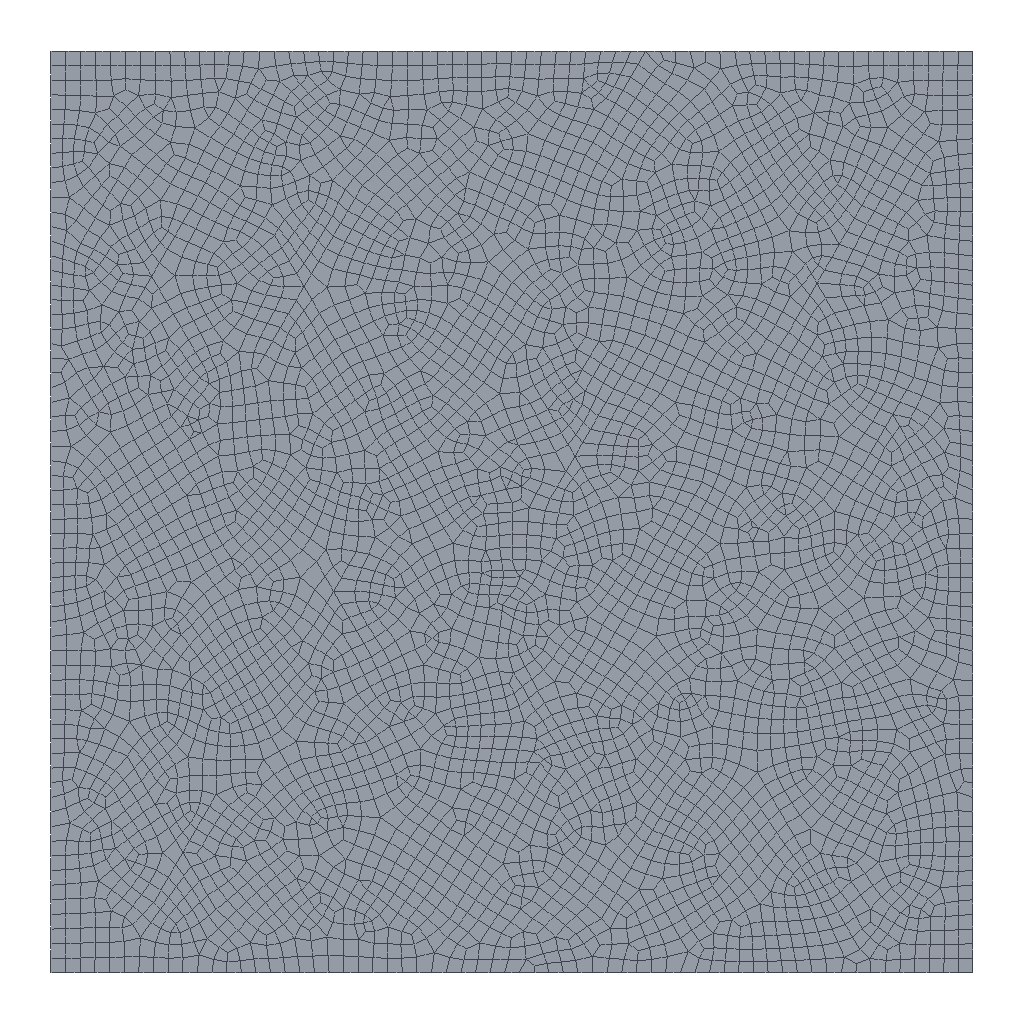Simulation study | abaqus
Notes in the study folder:
模型参数
尺寸 10cm*10cm
预制裂隙如cae
注入位置 和cae文件一样
渗透率 1e-16 m^2
孔隙度 3%
比热容 1.26 kJ/ （kg*K）
热导率 0.25 W/(m·K）
杨氏模量 3000MPa
泊松比 0.35
密度 1.3 g/cm^3

co2流体
 密度 0.5g / cm^3
 粘度 0.000026ps*s
滤失系数 10-3m/min^0.5
温度40℃


注入条件
40ml/min

加载条件
最小水平主应力 11MPa
最大水平主应力  15MPa

温度模型
骨架温度是40℃往中心传导
流体温度是40℃扩展过程中传导
Set-up summary:
category,name,step,type,value,unit,region
solver,abaqus
solver,version,,,Abaqus/Standard 3DEXPERIENCE R2017x
units,not stated in the deck,,not stated
analysis,deck,,thermal,thermal
load_step,Step-1,Step-1,thermal
load_step,requested,,,1
mesh,nodes,,,14396
mesh,elements,,,4771
element_type,DC2D6,,solid,169
element_type,DC2D8,,solid,4602
load,load commands in deck,,count,1
bc,support commands in deck,,count,1
material,MATERIAL-COHE1,,in results
material,MATERIAL-COHE2,,in results
material,MATERIAL-ROCK,,in results
check,setup vs results,,match,"per instance, exact: element labels, types and connectivity; labels of the nodes the elements use; coordinates of those nodes at SINGLE_PRECISION in 1 of 1 instance(s)"
Abaqus input file, long lists of numbers shortened:
*Heading
** Job name: Job-heat Model name: Model-1-heat
** Generated by: Abaqus/CAE 2017
*Preprint, echo=NO, model=NO, history=NO, contact=NO
**
** PARTS
**
*Part, name=Part-1
*Node
      1,   6.038,  -20.003
      2,   6.831,  -18.63
** (14394 more lines like these left out)
*Element, type=DC2D6
  1, 3448, 4577, 2339, 4814, 4815, 4816
  2, 2953, 2672,  379, 4817, 4818, 4819
** (167 more lines like these left out)
*Element, type=DC2D8
 170,  1737,  1236,   227,  1666,  5319,  5320,  5321,  5322
 171,  1237,  1738,  1651,   229,  5323,  5324,  5325,  5326
** (4600 more lines like these left out)
*Nset, nset=Set-5, generate
     1,  14396,      1
*Elset, elset=Set-5, generate
    1,  4771,     1
** Section: Section-rock
*Solid Section, elset=Set-5, material=Material-rock
,
*End Part
**
**
** ASSEMBLY
**
*Assembly, name=Assembly
**
*Instance, name=Part-1-1, part=Part-1
*End Instance
**
*Nset, nset=Set-6, instance=Part-1-1, generate
     1,  14396,      1
*Elset, elset=Set-6, instance=Part-1-1, generate
    1,  4771,     1
*Nset, nset=Set-7, instance=Part-1-1
   181,   182,   183,   184,   185,   186,   187,   188,   189,   190,   191,   192,   193,   194,   195,   196
   197,   198,   199,   200,   201,   202,   203,   204,   205,   206,   207,   208,   209,   210,   211,   212
** (30 more lines like these left out)
*Elset, elset=Set-7, instance=Part-1-1
  170,  171,  172,  179,  219,  220,  221,  222,  224,  227,  243,  245,  258,  259,  260,  262
  263,  264,  266,  279,  316,  327,  376,  377,  378,  388,  390,  425,  426,  427,  538,  539
** (14 more lines like these left out)
*End Assembly
*Amplitude, name=Amp-1
             0.,              0.,              1.,              1.
**
** MATERIALS
**
*Material, name=Material-cohe1
*Conductivity
 0.25,
*Damage Initiation, criterion=MAXS
 2e+06, 1e+07, 1e+07
*Damage Evolution, type=DISPLACEMENT
 0.001,
*Density
1300.,
*Elastic, type=TRACTION
 1.5e+10, 1.5e+10, 1.5e+10
*Expansion
 6e-06,
*Fluid Leakoff
 1e-14, 1e-14
*Gap Flow
 0.001,
*Specific Heat
 1.26e+09,
*Material, name=Material-cohe2
*Conductivity
 0.25,
*Damage Initiation, criterion=MAXS
 6e+06, 2e+07, 2e+07
*Damage Evolution, type=DISPLACEMENT
 0.001,
*Density
1300.,
*Elastic, type=TRACTION
 1.5e+10, 1.5e+10, 1.5e+10
*Expansion
 5e-06,
*Fluid Leakoff
 1e-14, 1e-14
*Gap Flow
 0.001,
*Specific Heat
 1.26e+09,
*Material, name=Material-rock
*Conductivity
 0.25,
*Density
1300.,
*Elastic
 1.5e+10, 0.25
*Expansion
 5e-06,
*Permeability, specific=9800.
 1e-07, 0.1
*Specific Heat
1260.,
**
** PHYSICAL CONSTANTS
**
*Physical Constants, absolute zero=-273., stefan boltzmann=5.67e-08
** ----------------------------------------------------------------
**
** STEP: Step-1
**
*Step, name=Step-1, nlgeom=NO, inc=10000
*Heat Transfer, end=PERIOD
5e+06, 5e+08, , ,
**
** BOUNDARY CONDITIONS
**
** Name: BC-4 Type: 温度
*Boundary
Set-7, 11, 11, 40.
**
** CONTROLS
**
*Controls, reset
*Controls, parameters=time incrementation
, , , , , , , 10, , ,
**
** OUTPUT REQUESTS
**
*Restart, write, frequency=0
**
** FIELD OUTPUT: F-Output-2
**
*Output, field
*Node Output
NT, RFL
*Element Output, directions=YES
HFL, TEMP
*Radiation Output
FTEMP,
*Output, history, frequency=0
*End Step
Results summary:
result,step,,partial,increments=0 time=0.0/500000000.0
result,analysis,,,thermal
result,last_loadstep,,,1
result,primary field,,,NT11